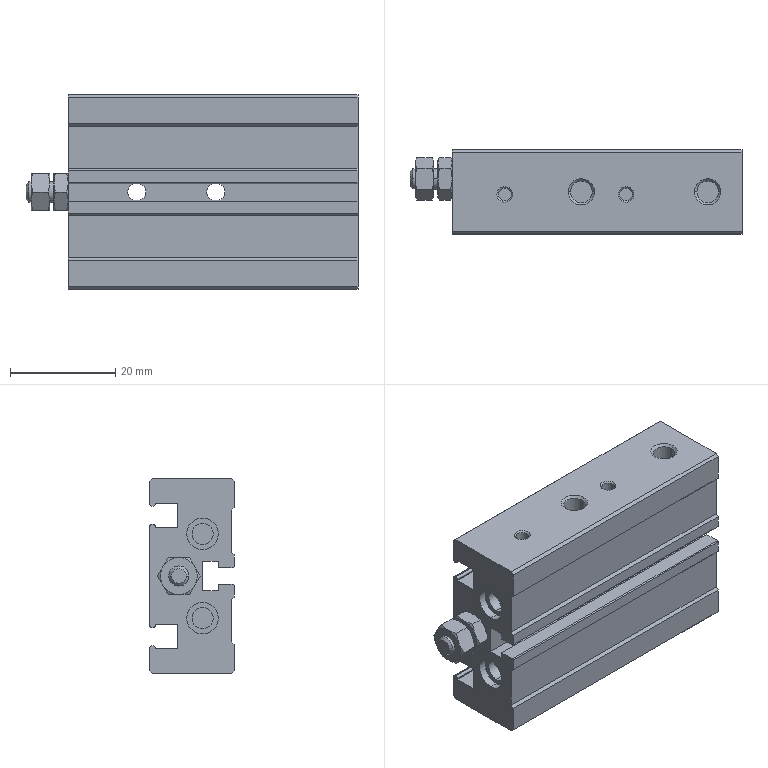Part | STEP file | _TR6-1010_b | 1 solid | 178 faces | box 63 x 16 x 37 mm | volume 25350 mm3 | plane 78 | cylinder 58 | cone 42 | commonest cylinder face diameters 0.8 x8 2.459 x8 4.134 x8 6 x8 4 x6 3.4 x4